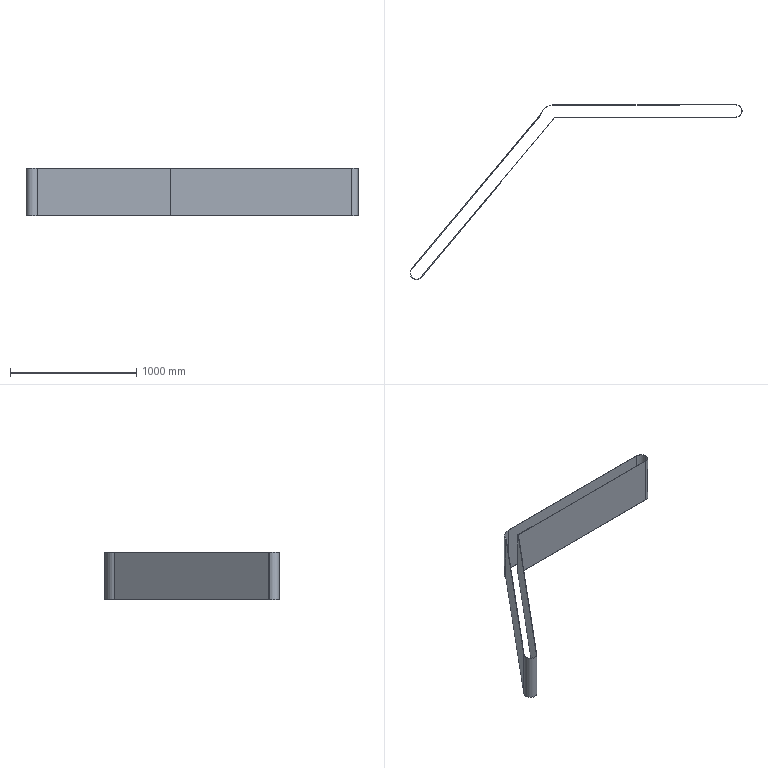Part | STEP file | Copy of PART1V11 | 1 solid | 18 faces | box 2633 x 1388 x 378 mm | volume 7453727 mm3 | plane 10 | cylinder 8 | commonest cylinder face diameters 97.16 x2 103.16 x2 97.182 x1 103.182 x1 212.439 x1 218.439 x1
STEP:
#1=CARTESIAN_POINT('',(0.,0.,0.));
#2=DIRECTION('',(0.,0.,1.));
#3=DIRECTION('',(1.,0.,0.));
#4=AXIS2_PLACEMENT_3D('',#1,#2,#3);
#5=CARTESIAN_POINT('',(472.127,652.827,-378.));
#6=VERTEX_POINT('',#5);
#7=CARTESIAN_POINT('',(472.127,652.827,0.));
#8=VERTEX_POINT('',#7);
#9=CARTESIAN_POINT('',(472.127,652.827,-378.));
#10=DIRECTION('',(0.,0.,1.));
#11=VECTOR('',#10,1.);
#12=LINE('',#9,#11);
#13=CARTESIAN_POINT('',(472.206,604.247,-378.));
#14=DIRECTION('',(0.,0.,1.));
#15=DIRECTION('',(1.,0.,0.));
#16=AXIS2_PLACEMENT_3D('',#13,#14,#15);
#17=CYLINDRICAL_SURFACE('',#16,48.58);
#18=CARTESIAN_POINT('',(1.572,0.));
#19=DIRECTION('',(0.,1.));
#20=VECTOR('',#19,1.);
#21=LINE('',#18,#20);
#22=(GEOMETRIC_REPRESENTATION_CONTEXT(2)PARAMETRIC_REPRESENTATION_CONTEXT()REPRESENTATION_CONTEXT('',''));
#23=DEFINITIONAL_REPRESENTATION('',(#21),#22);
#24=PCURVE('',#17,#23);
#25=CARTESIAN_POINT('',(472.127,652.827,-378.));
#26=DIRECTION('',(-0.001617,1.,0.));
#27=DIRECTION('',(-1.,-0.001617,0.));
#28=AXIS2_PLACEMENT_3D('',#25,#26,#27);
#29=PLANE('',#28);
#30=CARTESIAN_POINT('',(0.,0.));
#31=DIRECTION('',(0.,1.));
#32=VECTOR('',#31,1.);
#33=LINE('',#30,#32);
#34=(GEOMETRIC_REPRESENTATION_CONTEXT(2)PARAMETRIC_REPRESENTATION_CONTEXT()REPRESENTATION_CONTEXT('',''));
#35=DEFINITIONAL_REPRESENTATION('',(#33),#34);
#36=PCURVE('',#29,#35);
#37=SURFACE_CURVE('',#12,(#24,#36),.PCURVE_S1.);
#38=EDGE_CURVE('',#6,#8,#37,.T.);
#39=ORIENTED_EDGE('',*,*,#38,.T.);
#40=CARTESIAN_POINT('',(520.786,604.247,0.));
#41=VERTEX_POINT('',#40);
#42=CARTESIAN_POINT('',(472.206,604.247,0.));
#43=DIRECTION('',(0.,0.,1.));
#44=DIRECTION('',(1.,0.,0.));
#45=AXIS2_PLACEMENT_3D('',#42,#43,#44);
#46=CIRCLE('',#45,48.58);
#47=CARTESIAN_POINT('',(0.,378.));
#48=DIRECTION('',(1.,0.));
#49=VECTOR('',#48,1.);
#50=LINE('',#47,#49);
#51=(GEOMETRIC_REPRESENTATION_CONTEXT(2)PARAMETRIC_REPRESENTATION_CONTEXT()REPRESENTATION_CONTEXT('',''));
#52=DEFINITIONAL_REPRESENTATION('',(#50),#51);
#53=PCURVE('',#17,#52);
#54=CARTESIAN_POINT('',(-2057.802,-680.936,0.));
#55=DIRECTION('',(0.,0.,1.));
#56=DIRECTION('',(1.,0.,0.));
#57=AXIS2_PLACEMENT_3D('',#54,#55,#56);
#58=PLANE('',#57);
#59=CARTESIAN_POINT('',(2530.008,1285.182));
#60=DIRECTION('',(1.,0.));
#61=AXIS2_PLACEMENT_2D('',#59,#60);
#62=CIRCLE('',#61,48.58);
#63=(GEOMETRIC_REPRESENTATION_CONTEXT(2)PARAMETRIC_REPRESENTATION_CONTEXT()REPRESENTATION_CONTEXT('',''));
#64=DEFINITIONAL_REPRESENTATION('',(#62),#63);
#65=PCURVE('',#58,#64);
#66=SURFACE_CURVE('',#46,(#53,#65),.PCURVE_S1.);
#67=EDGE_CURVE('',#41,#8,#66,.T.);
#68=ORIENTED_EDGE('',*,*,#67,.F.);
#69=CARTESIAN_POINT('',(520.786,604.247,-378.));
#70=VERTEX_POINT('',#69);
#71=CARTESIAN_POINT('',(520.786,604.247,-378.));
#72=DIRECTION('',(0.,0.,1.));
#73=VECTOR('',#72,1.);
#74=LINE('',#71,#73);
#75=CARTESIAN_POINT('',(0.,0.));
#76=DIRECTION('',(0.,1.));
#77=VECTOR('',#76,1.);
#78=LINE('',#75,#77);
#79=(GEOMETRIC_REPRESENTATION_CONTEXT(2)PARAMETRIC_REPRESENTATION_CONTEXT()REPRESENTATION_CONTEXT('',''));
#80=DEFINITIONAL_REPRESENTATION('',(#78),#79);
#81=PCURVE('',#17,#80);
#82=CARTESIAN_POINT('',(472.206,604.247,-378.));
#83=DIRECTION('',(0.,0.,1.));
#84=DIRECTION('',(1.,0.,0.));
#85=AXIS2_PLACEMENT_3D('',#82,#83,#84);
#86=CYLINDRICAL_SURFACE('',#85,48.58);
#87=CARTESIAN_POINT('',(6.283,0.));
#88=DIRECTION('',(0.,1.));
#89=VECTOR('',#88,1.);
#90=LINE('',#87,#89);
#91=(GEOMETRIC_REPRESENTATION_CONTEXT(2)PARAMETRIC_REPRESENTATION_CONTEXT()REPRESENTATION_CONTEXT('',''));
#92=DEFINITIONAL_REPRESENTATION('',(#90),#91);
#93=PCURVE('',#86,#92);
#94=SURFACE_CURVE('',#74,(#81,#93),.PCURVE_S1.);
#95=EDGE_CURVE('',#70,#41,#94,.T.);
#96=ORIENTED_EDGE('',*,*,#95,.F.);
#97=CARTESIAN_POINT('',(472.206,604.247,-378.));
#98=DIRECTION('',(0.,0.,1.));
#99=DIRECTION('',(1.,0.,0.));
#100=AXIS2_PLACEMENT_3D('',#97,#98,#99);
#101=CIRCLE('',#100,48.58);
#102=CARTESIAN_POINT('',(0.,0.));
#103=DIRECTION('',(1.,0.));
#104=VECTOR('',#103,1.);
#105=LINE('',#102,#104);
#106=(GEOMETRIC_REPRESENTATION_CONTEXT(2)PARAMETRIC_REPRESENTATION_CONTEXT()REPRESENTATION_CONTEXT('',''));
#107=DEFINITIONAL_REPRESENTATION('',(#105),#106);
#108=PCURVE('',#17,#107);
#109=CARTESIAN_POINT('',(-2057.802,-680.936,-378.));
#110=DIRECTION('',(0.,0.,1.));
#111=DIRECTION('',(1.,0.,0.));
#112=AXIS2_PLACEMENT_3D('',#109,#110,#111);
#113=PLANE('',#112);
#114=CARTESIAN_POINT('',(2530.008,1285.182));
#115=DIRECTION('',(1.,0.));
#116=AXIS2_PLACEMENT_2D('',#114,#115);
#117=CIRCLE('',#116,48.58);
#118=(GEOMETRIC_REPRESENTATION_CONTEXT(2)PARAMETRIC_REPRESENTATION_CONTEXT()REPRESENTATION_CONTEXT('',''));
#119=DEFINITIONAL_REPRESENTATION('',(#117),#118);
#120=PCURVE('',#113,#119);
#121=SURFACE_CURVE('',#101,(#108,#120),.PCURVE_S1.);
#122=EDGE_CURVE('',#70,#6,#121,.T.);
#123=ORIENTED_EDGE('',*,*,#122,.T.);
#124=EDGE_LOOP('',(#39,#68,#96,#123));
#125=FACE_BOUND('',#124,.F.);
#126=ADVANCED_FACE('',(#125),#17,.F.);
#127=CARTESIAN_POINT('',(472.208,552.667,-378.));
#128=VERTEX_POINT('',#127);
#129=CARTESIAN_POINT('',(523.786,604.247,-378.));
#130=VERTEX_POINT('',#129);
#131=CARTESIAN_POINT('',(472.206,604.247,-378.));
#132=DIRECTION('',(0.,0.,1.));
#133=DIRECTION('',(1.,0.,0.));
#134=AXIS2_PLACEMENT_3D('',#131,#132,#133);
#135=CIRCLE('',#134,51.58);
#136=CARTESIAN_POINT('',(472.206,604.247,-378.));
#137=DIRECTION('',(0.,0.,1.));
#138=DIRECTION('',(1.,0.,0.));
#139=AXIS2_PLACEMENT_3D('',#136,#137,#138);
#140=CYLINDRICAL_SURFACE('',#139,51.58);
#141=CARTESIAN_POINT('',(0.,0.));
#142=DIRECTION('',(1.,0.));
#143=VECTOR('',#142,1.);
#144=LINE('',#141,#143);
#145=(GEOMETRIC_REPRESENTATION_CONTEXT(2)PARAMETRIC_REPRESENTATION_CONTEXT()REPRESENTATION_CONTEXT('',''));
#146=DEFINITIONAL_REPRESENTATION('',(#144),#145);
#147=PCURVE('',#140,#146);
#148=CARTESIAN_POINT('',(2530.008,1285.182));
#149=DIRECTION('',(1.,0.));
#150=AXIS2_PLACEMENT_2D('',#148,#149);
#151=CIRCLE('',#150,51.58);
#152=(GEOMETRIC_REPRESENTATION_CONTEXT(2)PARAMETRIC_REPRESENTATION_CONTEXT()REPRESENTATION_CONTEXT('',''));
#153=DEFINITIONAL_REPRESENTATION('',(#151),#152);
#154=PCURVE('',#113,#153);
#155=SURFACE_CURVE('',#135,(#147,#154),.PCURVE_S1.);
#156=EDGE_CURVE('',#128,#130,#155,.T.);
#157=ORIENTED_EDGE('',*,*,#156,.T.);
#158=CARTESIAN_POINT('',(523.786,604.247,0.));
#159=VERTEX_POINT('',#158);
#160=CARTESIAN_POINT('',(523.786,604.247,-378.));
#161=DIRECTION('',(0.,0.,1.));
#162=VECTOR('',#161,1.);
#163=LINE('',#160,#162);
#164=CARTESIAN_POINT('',(6.283,0.));
#165=DIRECTION('',(0.,1.));
#166=VECTOR('',#165,1.);
#167=LINE('',#164,#166);
#168=(GEOMETRIC_REPRESENTATION_CONTEXT(2)PARAMETRIC_REPRESENTATION_CONTEXT()REPRESENTATION_CONTEXT('',''));
#169=DEFINITIONAL_REPRESENTATION('',(#167),#168);
#170=PCURVE('',#140,#169);
#171=CARTESIAN_POINT('',(472.206,604.247,-378.));
#172=DIRECTION('',(0.,0.,1.));
#173=DIRECTION('',(1.,0.,0.));
#174=AXIS2_PLACEMENT_3D('',#171,#172,#173);
#175=CYLINDRICAL_SURFACE('',#174,51.58);
#176=CARTESIAN_POINT('',(0.,0.));
#177=DIRECTION('',(0.,1.));
#178=VECTOR('',#177,1.);
#179=LINE('',#176,#178);
#180=(GEOMETRIC_REPRESENTATION_CONTEXT(2)PARAMETRIC_REPRESENTATION_CONTEXT()REPRESENTATION_CONTEXT('',''));
#181=DEFINITIONAL_REPRESENTATION('',(#179),#180);
#182=PCURVE('',#175,#181);
#183=SURFACE_CURVE('',#163,(#170,#182),.PCURVE_S1.);
#184=EDGE_CURVE('',#130,#159,#183,.T.);
#185=ORIENTED_EDGE('',*,*,#184,.T.);
#186=CARTESIAN_POINT('',(472.208,552.667,0.));
#187=VERTEX_POINT('',#186);
#188=CARTESIAN_POINT('',(472.206,604.247,0.));
#189=DIRECTION('',(0.,0.,1.));
#190=DIRECTION('',(1.,0.,0.));
#191=AXIS2_PLACEMENT_3D('',#188,#189,#190);
#192=CIRCLE('',#191,51.58);
#193=CARTESIAN_POINT('',(0.,378.));
#194=DIRECTION('',(1.,0.));
#195=VECTOR('',#194,1.);
#196=LINE('',#193,#195);
#197=(GEOMETRIC_REPRESENTATION_CONTEXT(2)PARAMETRIC_REPRESENTATION_CONTEXT()REPRESENTATION_CONTEXT('',''));
#198=DEFINITIONAL_REPRESENTATION('',(#196),#197);
#199=PCURVE('',#140,#198);
#200=CARTESIAN_POINT('',(2530.008,1285.182));
#201=DIRECTION('',(1.,0.));
#202=AXIS2_PLACEMENT_2D('',#200,#201);
#203=CIRCLE('',#202,51.58);
#204=(GEOMETRIC_REPRESENTATION_CONTEXT(2)PARAMETRIC_REPRESENTATION_CONTEXT()REPRESENTATION_CONTEXT('',''));
#205=DEFINITIONAL_REPRESENTATION('',(#203),#204);
#206=PCURVE('',#58,#205);
#207=SURFACE_CURVE('',#192,(#199,#206),.PCURVE_S1.);
#208=EDGE_CURVE('',#187,#159,#207,.T.);
#209=ORIENTED_EDGE('',*,*,#208,.F.);
#210=CARTESIAN_POINT('',(472.208,552.667,-378.));
#211=DIRECTION('',(0.,0.,1.));
#212=VECTOR('',#211,1.);
#213=LINE('',#210,#212);
#214=CARTESIAN_POINT('',(4.712,0.));
#215=DIRECTION('',(0.,1.));
#216=VECTOR('',#215,1.);
#217=LINE('',#214,#216);
#218=(GEOMETRIC_REPRESENTATION_CONTEXT(2)PARAMETRIC_REPRESENTATION_CONTEXT()REPRESENTATION_CONTEXT('',''));
#219=DEFINITIONAL_REPRESENTATION('',(#217),#218);
#220=PCURVE('',#140,#219);
#221=CARTESIAN_POINT('',(472.208,552.667,-378.));
#222=DIRECTION('',(0.001617,-1.,0.));
#223=DIRECTION('',(1.,0.001617,0.));
#224=AXIS2_PLACEMENT_3D('',#221,#222,#223);
#225=PLANE('',#224);
#226=CARTESIAN_POINT('',(0.,0.));
#227=DIRECTION('',(0.,1.));
#228=VECTOR('',#227,1.);
#229=LINE('',#226,#228);
#230=(GEOMETRIC_REPRESENTATION_CONTEXT(2)PARAMETRIC_REPRESENTATION_CONTEXT()REPRESENTATION_CONTEXT('',''));
#231=DEFINITIONAL_REPRESENTATION('',(#229),#230);
#232=PCURVE('',#225,#231);
#233=SURFACE_CURVE('',#213,(#220,#232),.PCURVE_S1.);
#234=EDGE_CURVE('',#128,#187,#233,.T.);
#235=ORIENTED_EDGE('',*,*,#234,.F.);
#236=EDGE_LOOP('',(#157,#185,#209,#235));
#237=FACE_BOUND('',#236,.T.);
#238=ADVANCED_FACE('',(#237),#140,.T.);
#239=CARTESIAN_POINT('',(-2097.377,-647.838,0.));
#240=VERTEX_POINT('',#239);
#241=CARTESIAN_POINT('',(-2018.228,-714.034,0.));
#242=VERTEX_POINT('',#241);
#243=CARTESIAN_POINT('',(-2057.802,-680.936,0.));
#244=DIRECTION('',(0.,0.,1.));
#245=DIRECTION('',(1.,0.,0.));
#246=AXIS2_PLACEMENT_3D('',#243,#244,#245);
#247=CIRCLE('',#246,51.591);
#248=CARTESIAN_POINT('',(-2057.802,-680.936,-378.));
#249=DIRECTION('',(0.,0.,1.));
#250=DIRECTION('',(1.,0.,0.));
#251=AXIS2_PLACEMENT_3D('',#248,#249,#250);
#252=CYLINDRICAL_SURFACE('',#251,51.591);
#253=CARTESIAN_POINT('',(0.,378.));
#254=DIRECTION('',(1.,0.));
#255=VECTOR('',#254,1.);
#256=LINE('',#253,#255);
#257=(GEOMETRIC_REPRESENTATION_CONTEXT(2)PARAMETRIC_REPRESENTATION_CONTEXT()REPRESENTATION_CONTEXT('',''));
#258=DEFINITIONAL_REPRESENTATION('',(#256),#257);
#259=PCURVE('',#252,#258);
#260=CARTESIAN_POINT('',(0.,0.));
#261=DIRECTION('',(1.,0.));
#262=AXIS2_PLACEMENT_2D('',#260,#261);
#263=CIRCLE('',#262,51.591);
#264=(GEOMETRIC_REPRESENTATION_CONTEXT(2)PARAMETRIC_REPRESENTATION_CONTEXT()REPRESENTATION_CONTEXT('',''));
#265=DEFINITIONAL_REPRESENTATION('',(#263),#264);
#266=PCURVE('',#58,#265);
#267=SURFACE_CURVE('',#247,(#259,#266),.PCURVE_S1.);
#268=EDGE_CURVE('',#240,#242,#267,.T.);
#269=ORIENTED_EDGE('',*,*,#268,.F.);
#270=CARTESIAN_POINT('',(-2097.377,-647.838,-378.));
#271=VERTEX_POINT('',#270);
#272=CARTESIAN_POINT('',(-2097.377,-647.838,-378.));
#273=DIRECTION('',(0.,0.,1.));
#274=VECTOR('',#273,1.);
#275=LINE('',#272,#274);
#276=CARTESIAN_POINT('',(2.445,0.));
#277=DIRECTION('',(0.,1.));
#278=VECTOR('',#277,1.);
#279=LINE('',#276,#278);
#280=(GEOMETRIC_REPRESENTATION_CONTEXT(2)PARAMETRIC_REPRESENTATION_CONTEXT()REPRESENTATION_CONTEXT('',''));
#281=DEFINITIONAL_REPRESENTATION('',(#279),#280);
#282=PCURVE('',#252,#281);
#283=CARTESIAN_POINT('',(-2097.377,-647.838,-378.));
#284=DIRECTION('',(-0.7671,0.6415,0.));
#285=DIRECTION('',(-0.6415,-0.7671,0.));
#286=AXIS2_PLACEMENT_3D('',#283,#284,#285);
#287=PLANE('',#286);
#288=CARTESIAN_POINT('',(0.,0.));
#289=DIRECTION('',(0.,1.));
#290=VECTOR('',#289,1.);
#291=LINE('',#288,#290);
#292=(GEOMETRIC_REPRESENTATION_CONTEXT(2)PARAMETRIC_REPRESENTATION_CONTEXT()REPRESENTATION_CONTEXT('',''));
#293=DEFINITIONAL_REPRESENTATION('',(#291),#292);
#294=PCURVE('',#287,#293);
#295=SURFACE_CURVE('',#275,(#282,#294),.PCURVE_S1.);
#296=EDGE_CURVE('',#271,#240,#295,.T.);
#297=ORIENTED_EDGE('',*,*,#296,.F.);
#298=CARTESIAN_POINT('',(-2018.228,-714.034,-378.));
#299=VERTEX_POINT('',#298);
#300=CARTESIAN_POINT('',(-2057.802,-680.936,-378.));
#301=DIRECTION('',(0.,0.,1.));
#302=DIRECTION('',(1.,0.,0.));
#303=AXIS2_PLACEMENT_3D('',#300,#301,#302);
#304=CIRCLE('',#303,51.591);
#305=CARTESIAN_POINT('',(0.,0.));
#306=DIRECTION('',(1.,0.));
#307=VECTOR('',#306,1.);
#308=LINE('',#305,#307);
#309=(GEOMETRIC_REPRESENTATION_CONTEXT(2)PARAMETRIC_REPRESENTATION_CONTEXT()REPRESENTATION_CONTEXT('',''));
#310=DEFINITIONAL_REPRESENTATION('',(#308),#309);
#311=PCURVE('',#252,#310);
#312=CARTESIAN_POINT('',(0.,0.));
#313=DIRECTION('',(1.,0.));
#314=AXIS2_PLACEMENT_2D('',#312,#313);
#315=CIRCLE('',#314,51.591);
#316=(GEOMETRIC_REPRESENTATION_CONTEXT(2)PARAMETRIC_REPRESENTATION_CONTEXT()REPRESENTATION_CONTEXT('',''));
#317=DEFINITIONAL_REPRESENTATION('',(#315),#316);
#318=PCURVE('',#113,#317);
#319=SURFACE_CURVE('',#304,(#311,#318),.PCURVE_S1.);
#320=EDGE_CURVE('',#271,#299,#319,.T.);
#321=ORIENTED_EDGE('',*,*,#320,.T.);
#322=CARTESIAN_POINT('',(-2018.228,-714.034,-378.));
#323=DIRECTION('',(0.,0.,1.));
#324=VECTOR('',#323,1.);
#325=LINE('',#322,#324);
#326=CARTESIAN_POINT('',(5.587,0.));
#327=DIRECTION('',(0.,1.));
#328=VECTOR('',#327,1.);
#329=LINE('',#326,#328);
#330=(GEOMETRIC_REPRESENTATION_CONTEXT(2)PARAMETRIC_REPRESENTATION_CONTEXT()REPRESENTATION_CONTEXT('',''));
#331=DEFINITIONAL_REPRESENTATION('',(#329),#330);
#332=PCURVE('',#252,#331);
#333=CARTESIAN_POINT('',(-960.762,550.35,-378.));
#334=DIRECTION('',(0.7671,-0.6415,0.));
#335=DIRECTION('',(0.6415,0.7671,0.));
#336=AXIS2_PLACEMENT_3D('',#333,#334,#335);
#337=PLANE('',#336);
#338=CARTESIAN_POINT('',(-1648.303,0.));
#339=DIRECTION('',(0.,1.));
#340=VECTOR('',#339,1.);
#341=LINE('',#338,#340);
#342=(GEOMETRIC_REPRESENTATION_CONTEXT(2)PARAMETRIC_REPRESENTATION_CONTEXT()REPRESENTATION_CONTEXT('',''));
#343=DEFINITIONAL_REPRESENTATION('',(#341),#342);
#344=PCURVE('',#337,#343);
#345=SURFACE_CURVE('',#325,(#332,#344),.PCURVE_S1.);
#346=EDGE_CURVE('',#299,#242,#345,.T.);
#347=ORIENTED_EDGE('',*,*,#346,.T.);
#348=EDGE_LOOP('',(#269,#297,#321,#347));
#349=FACE_BOUND('',#348,.T.);
#350=ADVANCED_FACE('',(#349),#252,.T.);
#351=CARTESIAN_POINT('',(-1075.448,574.055,0.));
#352=VERTEX_POINT('',#351);
#353=CARTESIAN_POINT('',(-2097.377,-647.838,0.));
#354=DIRECTION('',(-0.6415,-0.7671,0.));
#355=VECTOR('',#354,1.);
#356=LINE('',#353,#355);
#357=CARTESIAN_POINT('',(0.,378.));
#358=DIRECTION('',(1.,0.));
#359=VECTOR('',#358,1.);
#360=LINE('',#357,#359);
#361=(GEOMETRIC_REPRESENTATION_CONTEXT(2)PARAMETRIC_REPRESENTATION_CONTEXT()REPRESENTATION_CONTEXT('',''));
#362=DEFINITIONAL_REPRESENTATION('',(#360),#361);
#363=PCURVE('',#287,#362);
#364=CARTESIAN_POINT('',(-39.574,33.098));
#365=DIRECTION('',(-0.6415,-0.7671));
#366=VECTOR('',#365,1.);
#367=LINE('',#364,#366);
#368=(GEOMETRIC_REPRESENTATION_CONTEXT(2)PARAMETRIC_REPRESENTATION_CONTEXT()REPRESENTATION_CONTEXT('',''));
#369=DEFINITIONAL_REPRESENTATION('',(#367),#368);
#370=PCURVE('',#58,#369);
#371=SURFACE_CURVE('',#356,(#363,#370),.PCURVE_S1.);
#372=EDGE_CURVE('',#352,#240,#371,.T.);
#373=ORIENTED_EDGE('',*,*,#372,.F.);
#374=CARTESIAN_POINT('',(-1075.448,574.055,-378.));
#375=VERTEX_POINT('',#374);
#376=CARTESIAN_POINT('',(-1075.448,574.055,-378.));
#377=DIRECTION('',(0.,0.,1.));
#378=VECTOR('',#377,1.);
#379=LINE('',#376,#378);
#380=CARTESIAN_POINT('',(-1592.909,0.));
#381=DIRECTION('',(0.,1.));
#382=VECTOR('',#381,1.);
#383=LINE('',#380,#382);
#384=(GEOMETRIC_REPRESENTATION_CONTEXT(2)PARAMETRIC_REPRESENTATION_CONTEXT()REPRESENTATION_CONTEXT('',''));
#385=DEFINITIONAL_REPRESENTATION('',(#383),#384);
#386=PCURVE('',#287,#385);
#387=CARTESIAN_POINT('',(-970.367,544.275,-378.));
#388=DIRECTION('',(0.,0.,1.));
#389=DIRECTION('',(1.,0.,0.));
#390=AXIS2_PLACEMENT_3D('',#387,#388,#389);
#391=CYLINDRICAL_SURFACE('',#390,109.22);
#392=CARTESIAN_POINT('',(2.865,0.));
#393=DIRECTION('',(0.,1.));
#394=VECTOR('',#393,1.);
#395=LINE('',#392,#394);
#396=(GEOMETRIC_REPRESENTATION_CONTEXT(2)PARAMETRIC_REPRESENTATION_CONTEXT()REPRESENTATION_CONTEXT('',''));
#397=DEFINITIONAL_REPRESENTATION('',(#395),#396);
#398=PCURVE('',#391,#397);
#399=SURFACE_CURVE('',#379,(#386,#398),.PCURVE_S1.);
#400=EDGE_CURVE('',#375,#352,#399,.T.);
#401=ORIENTED_EDGE('',*,*,#400,.F.);
#402=CARTESIAN_POINT('',(-2097.377,-647.838,-378.));
#403=DIRECTION('',(-0.6415,-0.7671,0.));
#404=VECTOR('',#403,1.);
#405=LINE('',#402,#404);
#406=CARTESIAN_POINT('',(0.,0.));
#407=DIRECTION('',(1.,0.));
#408=VECTOR('',#407,1.);
#409=LINE('',#406,#408);
#410=(GEOMETRIC_REPRESENTATION_CONTEXT(2)PARAMETRIC_REPRESENTATION_CONTEXT()REPRESENTATION_CONTEXT('',''));
#411=DEFINITIONAL_REPRESENTATION('',(#409),#410);
#412=PCURVE('',#287,#411);
#413=CARTESIAN_POINT('',(-39.574,33.098));
#414=DIRECTION('',(-0.6415,-0.7671));
#415=VECTOR('',#414,1.);
#416=LINE('',#413,#415);
#417=(GEOMETRIC_REPRESENTATION_CONTEXT(2)PARAMETRIC_REPRESENTATION_CONTEXT()REPRESENTATION_CONTEXT('',''));
#418=DEFINITIONAL_REPRESENTATION('',(#416),#417);
#419=PCURVE('',#113,#418);
#420=SURFACE_CURVE('',#405,(#412,#419),.PCURVE_S1.);
#421=EDGE_CURVE('',#375,#271,#420,.T.);
#422=ORIENTED_EDGE('',*,*,#421,.T.);
#423=ORIENTED_EDGE('',*,*,#296,.T.);
#424=EDGE_LOOP('',(#373,#401,#422,#423));
#425=FACE_BOUND('',#424,.T.);
#426=ADVANCED_FACE('',(#425),#287,.T.);
#427=CARTESIAN_POINT('',(-970.543,653.495,0.));
#428=VERTEX_POINT('',#427);
#429=CARTESIAN_POINT('',(-970.367,544.275,0.));
#430=DIRECTION('',(0.,0.,1.));
#431=DIRECTION('',(1.,0.,0.));
#432=AXIS2_PLACEMENT_3D('',#429,#430,#431);
#433=CIRCLE('',#432,109.22);
#434=CARTESIAN_POINT('',(0.,378.));
#435=DIRECTION('',(1.,0.));
#436=VECTOR('',#435,1.);
#437=LINE('',#434,#436);
#438=(GEOMETRIC_REPRESENTATION_CONTEXT(2)PARAMETRIC_REPRESENTATION_CONTEXT()REPRESENTATION_CONTEXT('',''));
#439=DEFINITIONAL_REPRESENTATION('',(#437),#438);
#440=PCURVE('',#391,#439);
#441=CARTESIAN_POINT('',(1087.435,1225.211));
#442=DIRECTION('',(1.,0.));
#443=AXIS2_PLACEMENT_2D('',#441,#442);
#444=CIRCLE('',#443,109.22);
#445=(GEOMETRIC_REPRESENTATION_CONTEXT(2)PARAMETRIC_REPRESENTATION_CONTEXT()REPRESENTATION_CONTEXT('',''));
#446=DEFINITIONAL_REPRESENTATION('',(#444),#445);
#447=PCURVE('',#58,#446);
#448=SURFACE_CURVE('',#433,(#440,#447),.PCURVE_S1.);
#449=EDGE_CURVE('',#428,#352,#448,.T.);
#450=ORIENTED_EDGE('',*,*,#449,.F.);
#451=CARTESIAN_POINT('',(-970.543,653.495,-378.));
#452=VERTEX_POINT('',#451);
#453=CARTESIAN_POINT('',(-970.543,653.495,-378.));
#454=DIRECTION('',(0.,0.,1.));
#455=VECTOR('',#454,1.);
#456=LINE('',#453,#455);
#457=CARTESIAN_POINT('',(1.572,0.));
#458=DIRECTION('',(0.,1.));
#459=VECTOR('',#458,1.);
#460=LINE('',#457,#459);
#461=(GEOMETRIC_REPRESENTATION_CONTEXT(2)PARAMETRIC_REPRESENTATION_CONTEXT()REPRESENTATION_CONTEXT('',''));
#462=DEFINITIONAL_REPRESENTATION('',(#460),#461);
#463=PCURVE('',#391,#462);
#464=CARTESIAN_POINT('',(472.122,655.827,-378.));
#465=DIRECTION('',(-0.001617,1.,0.));
#466=DIRECTION('',(-1.,-0.001617,0.));
#467=AXIS2_PLACEMENT_3D('',#464,#465,#466);
#468=PLANE('',#467);
#469=CARTESIAN_POINT('',(1442.668,0.));
#470=DIRECTION('',(0.,1.));
#471=VECTOR('',#470,1.);
#472=LINE('',#469,#471);
#473=(GEOMETRIC_REPRESENTATION_CONTEXT(2)PARAMETRIC_REPRESENTATION_CONTEXT()REPRESENTATION_CONTEXT('',''));
#474=DEFINITIONAL_REPRESENTATION('',(#472),#473);
#475=PCURVE('',#468,#474);
#476=SURFACE_CURVE('',#456,(#463,#475),.PCURVE_S1.);
#477=EDGE_CURVE('',#452,#428,#476,.T.);
#478=ORIENTED_EDGE('',*,*,#477,.F.);
#479=CARTESIAN_POINT('',(-970.367,544.275,-378.));
#480=DIRECTION('',(0.,0.,1.));
#481=DIRECTION('',(1.,0.,0.));
#482=AXIS2_PLACEMENT_3D('',#479,#480,#481);
#483=CIRCLE('',#482,109.22);
#484=CARTESIAN_POINT('',(0.,0.));
#485=DIRECTION('',(1.,0.));
#486=VECTOR('',#485,1.);
#487=LINE('',#484,#486);
#488=(GEOMETRIC_REPRESENTATION_CONTEXT(2)PARAMETRIC_REPRESENTATION_CONTEXT()REPRESENTATION_CONTEXT('',''));
#489=DEFINITIONAL_REPRESENTATION('',(#487),#488);
#490=PCURVE('',#391,#489);
#491=CARTESIAN_POINT('',(1087.435,1225.211));
#492=DIRECTION('',(1.,0.));
#493=AXIS2_PLACEMENT_2D('',#491,#492);
#494=CIRCLE('',#493,109.22);
#495=(GEOMETRIC_REPRESENTATION_CONTEXT(2)PARAMETRIC_REPRESENTATION_CONTEXT()REPRESENTATION_CONTEXT('',''));
#496=DEFINITIONAL_REPRESENTATION('',(#494),#495);
#497=PCURVE('',#113,#496);
#498=SURFACE_CURVE('',#483,(#490,#497),.PCURVE_S1.);
#499=EDGE_CURVE('',#452,#375,#498,.T.);
#500=ORIENTED_EDGE('',*,*,#499,.T.);
#501=ORIENTED_EDGE('',*,*,#400,.T.);
#502=EDGE_LOOP('',(#450,#478,#500,#501));
#503=FACE_BOUND('',#502,.T.);
#504=ADVANCED_FACE('',(#503),#391,.T.);
#505=CARTESIAN_POINT('',(472.122,655.827,0.));
#506=VERTEX_POINT('',#505);
#507=CARTESIAN_POINT('',(472.122,655.827,0.));
#508=DIRECTION('',(-1.,-0.001617,0.));
#509=VECTOR('',#508,1.);
#510=LINE('',#507,#509);
#511=CARTESIAN_POINT('',(0.,378.));
#512=DIRECTION('',(1.,0.));
#513=VECTOR('',#512,1.);
#514=LINE('',#511,#513);
#515=(GEOMETRIC_REPRESENTATION_CONTEXT(2)PARAMETRIC_REPRESENTATION_CONTEXT()REPRESENTATION_CONTEXT('',''));
#516=DEFINITIONAL_REPRESENTATION('',(#514),#515);
#517=PCURVE('',#468,#516);
#518=CARTESIAN_POINT('',(2529.925,1336.762));
#519=DIRECTION('',(-1.,-0.001617));
#520=VECTOR('',#519,1.);
#521=LINE('',#518,#520);
#522=(GEOMETRIC_REPRESENTATION_CONTEXT(2)PARAMETRIC_REPRESENTATION_CONTEXT()REPRESENTATION_CONTEXT('',''));
#523=DEFINITIONAL_REPRESENTATION('',(#521),#522);
#524=PCURVE('',#58,#523);
#525=SURFACE_CURVE('',#510,(#517,#524),.PCURVE_S1.);
#526=EDGE_CURVE('',#506,#428,#525,.T.);
#527=ORIENTED_EDGE('',*,*,#526,.F.);
#528=CARTESIAN_POINT('',(472.122,655.827,-378.));
#529=VERTEX_POINT('',#528);
#530=CARTESIAN_POINT('',(472.122,655.827,-378.));
#531=DIRECTION('',(0.,0.,1.));
#532=VECTOR('',#531,1.);
#533=LINE('',#530,#532);
#534=CARTESIAN_POINT('',(0.,0.));
#535=DIRECTION('',(0.,1.));
#536=VECTOR('',#535,1.);
#537=LINE('',#534,#536);
#538=(GEOMETRIC_REPRESENTATION_CONTEXT(2)PARAMETRIC_REPRESENTATION_CONTEXT()REPRESENTATION_CONTEXT('',''));
#539=DEFINITIONAL_REPRESENTATION('',(#537),#538);
#540=PCURVE('',#468,#539);
#541=CARTESIAN_POINT('',(1.572,0.));
#542=DIRECTION('',(0.,1.));
#543=VECTOR('',#542,1.);
#544=LINE('',#541,#543);
#545=(GEOMETRIC_REPRESENTATION_CONTEXT(2)PARAMETRIC_REPRESENTATION_CONTEXT()REPRESENTATION_CONTEXT('',''));
#546=DEFINITIONAL_REPRESENTATION('',(#544),#545);
#547=PCURVE('',#175,#546);
#548=SURFACE_CURVE('',#533,(#540,#547),.PCURVE_S1.);
#549=EDGE_CURVE('',#529,#506,#548,.T.);
#550=ORIENTED_EDGE('',*,*,#549,.F.);
#551=CARTESIAN_POINT('',(472.122,655.827,-378.));
#552=DIRECTION('',(-1.,-0.001617,0.));
#553=VECTOR('',#552,1.);
#554=LINE('',#551,#553);
#555=CARTESIAN_POINT('',(0.,0.));
#556=DIRECTION('',(1.,0.));
#557=VECTOR('',#556,1.);
#558=LINE('',#555,#557);
#559=(GEOMETRIC_REPRESENTATION_CONTEXT(2)PARAMETRIC_REPRESENTATION_CONTEXT()REPRESENTATION_CONTEXT('',''));
#560=DEFINITIONAL_REPRESENTATION('',(#558),#559);
#561=PCURVE('',#468,#560);
#562=CARTESIAN_POINT('',(2529.925,1336.762));
#563=DIRECTION('',(-1.,-0.001617));
#564=VECTOR('',#563,1.);
#565=LINE('',#562,#564);
#566=(GEOMETRIC_REPRESENTATION_CONTEXT(2)PARAMETRIC_REPRESENTATION_CONTEXT()REPRESENTATION_CONTEXT('',''));
#567=DEFINITIONAL_REPRESENTATION('',(#565),#566);
#568=PCURVE('',#113,#567);
#569=SURFACE_CURVE('',#554,(#561,#568),.PCURVE_S1.);
#570=EDGE_CURVE('',#529,#452,#569,.T.);
#571=ORIENTED_EDGE('',*,*,#570,.T.);
#572=ORIENTED_EDGE('',*,*,#477,.T.);
#573=EDGE_LOOP('',(#527,#550,#571,#572));
#574=FACE_BOUND('',#573,.T.);
#575=ADVANCED_FACE('',(#574),#468,.T.);
#576=ORIENTED_EDGE('',*,*,#184,.F.);
#577=CARTESIAN_POINT('',(472.206,604.247,-378.));
#578=DIRECTION('',(0.,0.,1.));
#579=DIRECTION('',(1.,0.,0.));
#580=AXIS2_PLACEMENT_3D('',#577,#578,#579);
#581=CIRCLE('',#580,51.58);
#582=CARTESIAN_POINT('',(0.,0.));
#583=DIRECTION('',(1.,0.));
#584=VECTOR('',#583,1.);
#585=LINE('',#582,#584);
#586=(GEOMETRIC_REPRESENTATION_CONTEXT(2)PARAMETRIC_REPRESENTATION_CONTEXT()REPRESENTATION_CONTEXT('',''));
#587=DEFINITIONAL_REPRESENTATION('',(#585),#586);
#588=PCURVE('',#175,#587);
#589=CARTESIAN_POINT('',(2530.008,1285.182));
#590=DIRECTION('',(1.,0.));
#591=AXIS2_PLACEMENT_2D('',#589,#590);
#592=CIRCLE('',#591,51.58);
#593=(GEOMETRIC_REPRESENTATION_CONTEXT(2)PARAMETRIC_REPRESENTATION_CONTEXT()REPRESENTATION_CONTEXT('',''));
#594=DEFINITIONAL_REPRESENTATION('',(#592),#593);
#595=PCURVE('',#113,#594);
#596=SURFACE_CURVE('',#581,(#588,#595),.PCURVE_S1.);
#597=EDGE_CURVE('',#130,#529,#596,.T.);
#598=ORIENTED_EDGE('',*,*,#597,.T.);
#599=ORIENTED_EDGE('',*,*,#549,.T.);
#600=CARTESIAN_POINT('',(472.206,604.247,0.));
#601=DIRECTION('',(0.,0.,1.));
#602=DIRECTION('',(1.,0.,0.));
#603=AXIS2_PLACEMENT_3D('',#600,#601,#602);
#604=CIRCLE('',#603,51.58);
#605=CARTESIAN_POINT('',(0.,378.));
#606=DIRECTION('',(1.,0.));
#607=VECTOR('',#606,1.);
#608=LINE('',#605,#607);
#609=(GEOMETRIC_REPRESENTATION_CONTEXT(2)PARAMETRIC_REPRESENTATION_CONTEXT()REPRESENTATION_CONTEXT('',''));
#610=DEFINITIONAL_REPRESENTATION('',(#608),#609);
#611=PCURVE('',#175,#610);
#612=CARTESIAN_POINT('',(2530.008,1285.182));
#613=DIRECTION('',(1.,0.));
#614=AXIS2_PLACEMENT_2D('',#612,#613);
#615=CIRCLE('',#614,51.58);
#616=(GEOMETRIC_REPRESENTATION_CONTEXT(2)PARAMETRIC_REPRESENTATION_CONTEXT()REPRESENTATION_CONTEXT('',''));
#617=DEFINITIONAL_REPRESENTATION('',(#615),#616);
#618=PCURVE('',#58,#617);
#619=SURFACE_CURVE('',#604,(#611,#618),.PCURVE_S1.);
#620=EDGE_CURVE('',#159,#506,#619,.T.);
#621=ORIENTED_EDGE('',*,*,#620,.F.);
#622=EDGE_LOOP('',(#576,#598,#599,#621));
#623=FACE_BOUND('',#622,.T.);
#624=ADVANCED_FACE('',(#623),#175,.T.);
#625=CARTESIAN_POINT('',(-960.762,550.35,0.));
#626=VERTEX_POINT('',#625);
#627=CARTESIAN_POINT('',(472.208,552.667,0.));
#628=DIRECTION('',(1.,0.001617,0.));
#629=VECTOR('',#628,1.);
#630=LINE('',#627,#629);
#631=CARTESIAN_POINT('',(0.,378.));
#632=DIRECTION('',(1.,0.));
#633=VECTOR('',#632,1.);
#634=LINE('',#631,#633);
#635=(GEOMETRIC_REPRESENTATION_CONTEXT(2)PARAMETRIC_REPRESENTATION_CONTEXT()REPRESENTATION_CONTEXT('',''));
#636=DEFINITIONAL_REPRESENTATION('',(#634),#635);
#637=PCURVE('',#225,#636);
#638=CARTESIAN_POINT('',(2530.01,1233.602));
#639=DIRECTION('',(1.,0.001617));
#640=VECTOR('',#639,1.);
#641=LINE('',#638,#640);
#642=(GEOMETRIC_REPRESENTATION_CONTEXT(2)PARAMETRIC_REPRESENTATION_CONTEXT()REPRESENTATION_CONTEXT('',''));
#643=DEFINITIONAL_REPRESENTATION('',(#641),#642);
#644=PCURVE('',#58,#643);
#645=SURFACE_CURVE('',#630,(#637,#644),.PCURVE_S1.);
#646=EDGE_CURVE('',#626,#187,#645,.T.);
#647=ORIENTED_EDGE('',*,*,#646,.F.);
#648=CARTESIAN_POINT('',(-960.762,550.35,-378.));
#649=VERTEX_POINT('',#648);
#650=CARTESIAN_POINT('',(-960.762,550.35,-378.));
#651=DIRECTION('',(0.,0.,1.));
#652=VECTOR('',#651,1.);
#653=LINE('',#650,#652);
#654=CARTESIAN_POINT('',(-1432.972,0.));
#655=DIRECTION('',(0.,1.));
#656=VECTOR('',#655,1.);
#657=LINE('',#654,#656);
#658=(GEOMETRIC_REPRESENTATION_CONTEXT(2)PARAMETRIC_REPRESENTATION_CONTEXT()REPRESENTATION_CONTEXT('',''));
#659=DEFINITIONAL_REPRESENTATION('',(#657),#658);
#660=PCURVE('',#225,#659);
#661=CARTESIAN_POINT('',(0.,0.));
#662=DIRECTION('',(0.,1.));
#663=VECTOR('',#662,1.);
#664=LINE('',#661,#663);
#665=(GEOMETRIC_REPRESENTATION_CONTEXT(2)PARAMETRIC_REPRESENTATION_CONTEXT()REPRESENTATION_CONTEXT('',''));
#666=DEFINITIONAL_REPRESENTATION('',(#664),#665);
#667=PCURVE('',#337,#666);
#668=SURFACE_CURVE('',#653,(#660,#667),.PCURVE_S1.);
#669=EDGE_CURVE('',#649,#626,#668,.T.);
#670=ORIENTED_EDGE('',*,*,#669,.F.);
#671=CARTESIAN_POINT('',(472.208,552.667,-378.));
#672=DIRECTION('',(1.,0.001617,0.));
#673=VECTOR('',#672,1.);
#674=LINE('',#671,#673);
#675=CARTESIAN_POINT('',(0.,0.));
#676=DIRECTION('',(1.,0.));
#677=VECTOR('',#676,1.);
#678=LINE('',#675,#677);
#679=(GEOMETRIC_REPRESENTATION_CONTEXT(2)PARAMETRIC_REPRESENTATION_CONTEXT()REPRESENTATION_CONTEXT('',''));
#680=DEFINITIONAL_REPRESENTATION('',(#678),#679);
#681=PCURVE('',#225,#680);
#682=CARTESIAN_POINT('',(2530.01,1233.602));
#683=DIRECTION('',(1.,0.001617));
#684=VECTOR('',#683,1.);
#685=LINE('',#682,#684);
#686=(GEOMETRIC_REPRESENTATION_CONTEXT(2)PARAMETRIC_REPRESENTATION_CONTEXT()REPRESENTATION_CONTEXT('',''));
#687=DEFINITIONAL_REPRESENTATION('',(#685),#686);
#688=PCURVE('',#113,#687);
#689=SURFACE_CURVE('',#674,(#681,#688),.PCURVE_S1.);
#690=EDGE_CURVE('',#649,#128,#689,.T.);
#691=ORIENTED_EDGE('',*,*,#690,.T.);
#692=ORIENTED_EDGE('',*,*,#234,.T.);
#693=EDGE_LOOP('',(#647,#670,#691,#692));
#694=FACE_BOUND('',#693,.T.);
#695=ADVANCED_FACE('',(#694),#225,.T.);
#696=CARTESIAN_POINT('',(-960.762,550.35,0.));
#697=DIRECTION('',(0.6415,0.7671,0.));
#698=VECTOR('',#697,1.);
#699=LINE('',#696,#698);
#700=CARTESIAN_POINT('',(0.,378.));
#701=DIRECTION('',(1.,0.));
#702=VECTOR('',#701,1.);
#703=LINE('',#700,#702);
#704=(GEOMETRIC_REPRESENTATION_CONTEXT(2)PARAMETRIC_REPRESENTATION_CONTEXT()REPRESENTATION_CONTEXT('',''));
#705=DEFINITIONAL_REPRESENTATION('',(#703),#704);
#706=PCURVE('',#337,#705);
#707=CARTESIAN_POINT('',(1097.04,1231.286));
#708=DIRECTION('',(0.6415,0.7671));
#709=VECTOR('',#708,1.);
#710=LINE('',#707,#709);
#711=(GEOMETRIC_REPRESENTATION_CONTEXT(2)PARAMETRIC_REPRESENTATION_CONTEXT()REPRESENTATION_CONTEXT('',''));
#712=DEFINITIONAL_REPRESENTATION('',(#710),#711);
#713=PCURVE('',#58,#712);
#714=SURFACE_CURVE('',#699,(#706,#713),.PCURVE_S1.);
#715=EDGE_CURVE('',#242,#626,#714,.T.);
#716=ORIENTED_EDGE('',*,*,#715,.F.);
#717=ORIENTED_EDGE('',*,*,#346,.F.);
#718=CARTESIAN_POINT('',(-960.762,550.35,-378.));
#719=DIRECTION('',(0.6415,0.7671,0.));
#720=VECTOR('',#719,1.);
#721=LINE('',#718,#720);
#722=CARTESIAN_POINT('',(0.,0.));
#723=DIRECTION('',(1.,0.));
#724=VECTOR('',#723,1.);
#725=LINE('',#722,#724);
#726=(GEOMETRIC_REPRESENTATION_CONTEXT(2)PARAMETRIC_REPRESENTATION_CONTEXT()REPRESENTATION_CONTEXT('',''));
#727=DEFINITIONAL_REPRESENTATION('',(#725),#726);
#728=PCURVE('',#337,#727);
#729=CARTESIAN_POINT('',(1097.04,1231.286));
#730=DIRECTION('',(0.6415,0.7671));
#731=VECTOR('',#730,1.);
#732=LINE('',#729,#731);
#733=(GEOMETRIC_REPRESENTATION_CONTEXT(2)PARAMETRIC_REPRESENTATION_CONTEXT()REPRESENTATION_CONTEXT('',''));
#734=DEFINITIONAL_REPRESENTATION('',(#732),#733);
#735=PCURVE('',#113,#734);
#736=SURFACE_CURVE('',#721,(#728,#735),.PCURVE_S1.);
#737=EDGE_CURVE('',#299,#649,#736,.T.);
#738=ORIENTED_EDGE('',*,*,#737,.T.);
#739=ORIENTED_EDGE('',*,*,#669,.T.);
#740=EDGE_LOOP('',(#716,#717,#738,#739));
#741=FACE_BOUND('',#740,.T.);
#742=ADVANCED_FACE('',(#741),#337,.T.);
#743=CARTESIAN_POINT('',(-2020.529,-712.109,-378.));
#744=VERTEX_POINT('',#743);
#745=CARTESIAN_POINT('',(-962.166,553.348,-378.));
#746=VERTEX_POINT('',#745);
#747=CARTESIAN_POINT('',(-962.166,553.348,-378.));
#748=DIRECTION('',(0.6415,0.7671,0.));
#749=VECTOR('',#748,1.);
#750=LINE('',#747,#749);
#751=CARTESIAN_POINT('',(1095.637,1234.284));
#752=DIRECTION('',(0.6415,0.7671));
#753=VECTOR('',#752,1.);
#754=LINE('',#751,#753);
#755=(GEOMETRIC_REPRESENTATION_CONTEXT(2)PARAMETRIC_REPRESENTATION_CONTEXT()REPRESENTATION_CONTEXT('',''));
#756=DEFINITIONAL_REPRESENTATION('',(#754),#755);
#757=PCURVE('',#113,#756);
#758=CARTESIAN_POINT('',(-962.166,553.348,-378.));
#759=DIRECTION('',(0.7671,-0.6415,0.));
#760=DIRECTION('',(0.6415,0.7671,0.));
#761=AXIS2_PLACEMENT_3D('',#758,#759,#760);
#762=PLANE('',#761);
#763=CARTESIAN_POINT('',(0.,0.));
#764=DIRECTION('',(1.,0.));
#765=VECTOR('',#764,1.);
#766=LINE('',#763,#765);
#767=(GEOMETRIC_REPRESENTATION_CONTEXT(2)PARAMETRIC_REPRESENTATION_CONTEXT()REPRESENTATION_CONTEXT('',''));
#768=DEFINITIONAL_REPRESENTATION('',(#766),#767);
#769=PCURVE('',#762,#768);
#770=SURFACE_CURVE('',#750,(#757,#769),.PCURVE_S1.);
#771=EDGE_CURVE('',#744,#746,#770,.T.);
#772=ORIENTED_EDGE('',*,*,#771,.T.);
#773=CARTESIAN_POINT('',(472.206,555.667,-378.));
#774=VERTEX_POINT('',#773);
#775=CARTESIAN_POINT('',(472.206,555.667,-378.));
#776=DIRECTION('',(1.,0.001617,0.));
#777=VECTOR('',#776,1.);
#778=LINE('',#775,#777);
#779=CARTESIAN_POINT('',(2530.008,1236.602));
#780=DIRECTION('',(1.,0.001617));
#781=VECTOR('',#780,1.);
#782=LINE('',#779,#781);
#783=(GEOMETRIC_REPRESENTATION_CONTEXT(2)PARAMETRIC_REPRESENTATION_CONTEXT()REPRESENTATION_CONTEXT('',''));
#784=DEFINITIONAL_REPRESENTATION('',(#782),#783);
#785=PCURVE('',#113,#784);
#786=CARTESIAN_POINT('',(472.206,555.667,-378.));
#787=DIRECTION('',(0.001617,-1.,0.));
#788=DIRECTION('',(1.,0.001617,0.));
#789=AXIS2_PLACEMENT_3D('',#786,#787,#788);
#790=PLANE('',#789);
#791=CARTESIAN_POINT('',(0.,0.));
#792=DIRECTION('',(1.,0.));
#793=VECTOR('',#792,1.);
#794=LINE('',#791,#793);
#795=(GEOMETRIC_REPRESENTATION_CONTEXT(2)PARAMETRIC_REPRESENTATION_CONTEXT()REPRESENTATION_CONTEXT('',''));
#796=DEFINITIONAL_REPRESENTATION('',(#794),#795);
#797=PCURVE('',#790,#796);
#798=SURFACE_CURVE('',#778,(#785,#797),.PCURVE_S1.);
#799=EDGE_CURVE('',#746,#774,#798,.T.);
#800=ORIENTED_EDGE('',*,*,#799,.T.);
#801=CARTESIAN_POINT('',(472.206,604.247,-378.));
#802=DIRECTION('',(0.,0.,1.));
#803=DIRECTION('',(1.,0.,0.));
#804=AXIS2_PLACEMENT_3D('',#801,#802,#803);
#805=CIRCLE('',#804,48.58);
#806=CARTESIAN_POINT('',(2530.008,1285.182));
#807=DIRECTION('',(1.,0.));
#808=AXIS2_PLACEMENT_2D('',#806,#807);
#809=CIRCLE('',#808,48.58);
#810=(GEOMETRIC_REPRESENTATION_CONTEXT(2)PARAMETRIC_REPRESENTATION_CONTEXT()REPRESENTATION_CONTEXT('',''));
#811=DEFINITIONAL_REPRESENTATION('',(#809),#810);
#812=PCURVE('',#113,#811);
#813=CARTESIAN_POINT('',(0.,0.));
#814=DIRECTION('',(1.,0.));
#815=VECTOR('',#814,1.);
#816=LINE('',#813,#815);
#817=(GEOMETRIC_REPRESENTATION_CONTEXT(2)PARAMETRIC_REPRESENTATION_CONTEXT()REPRESENTATION_CONTEXT('',''));
#818=DEFINITIONAL_REPRESENTATION('',(#816),#817);
#819=PCURVE('',#86,#818);
#820=SURFACE_CURVE('',#805,(#812,#819),.PCURVE_S1.);
#821=EDGE_CURVE('',#774,#70,#820,.T.);
#822=ORIENTED_EDGE('',*,*,#821,.T.);
#823=ORIENTED_EDGE('',*,*,#122,.T.);
#824=CARTESIAN_POINT('',(-970.539,650.495,-378.));
#825=VERTEX_POINT('',#824);
#826=CARTESIAN_POINT('',(472.127,652.827,-378.));
#827=DIRECTION('',(-1.,-0.001617,0.));
#828=VECTOR('',#827,1.);
#829=LINE('',#826,#828);
#830=CARTESIAN_POINT('',(2529.929,1333.762));
#831=DIRECTION('',(-1.,-0.001617));
#832=VECTOR('',#831,1.);
#833=LINE('',#830,#832);
#834=(GEOMETRIC_REPRESENTATION_CONTEXT(2)PARAMETRIC_REPRESENTATION_CONTEXT()REPRESENTATION_CONTEXT('',''));
#835=DEFINITIONAL_REPRESENTATION('',(#833),#834);
#836=PCURVE('',#113,#835);
#837=CARTESIAN_POINT('',(0.,0.));
#838=DIRECTION('',(1.,0.));
#839=VECTOR('',#838,1.);
#840=LINE('',#837,#839);
#841=(GEOMETRIC_REPRESENTATION_CONTEXT(2)PARAMETRIC_REPRESENTATION_CONTEXT()REPRESENTATION_CONTEXT('',''));
#842=DEFINITIONAL_REPRESENTATION('',(#840),#841);
#843=PCURVE('',#29,#842);
#844=SURFACE_CURVE('',#829,(#836,#843),.PCURVE_S1.);
#845=EDGE_CURVE('',#6,#825,#844,.T.);
#846=ORIENTED_EDGE('',*,*,#845,.T.);
#847=CARTESIAN_POINT('',(-1072.733,572.625,-378.));
#848=VERTEX_POINT('',#847);
#849=CARTESIAN_POINT('',(-970.367,544.275,-378.));
#850=DIRECTION('',(0.,0.,1.));
#851=DIRECTION('',(1.,0.,0.));
#852=AXIS2_PLACEMENT_3D('',#849,#850,#851);
#853=CIRCLE('',#852,106.22);
#854=CARTESIAN_POINT('',(1087.435,1225.211));
#855=DIRECTION('',(1.,0.));
#856=AXIS2_PLACEMENT_2D('',#854,#855);
#857=CIRCLE('',#856,106.22);
#858=(GEOMETRIC_REPRESENTATION_CONTEXT(2)PARAMETRIC_REPRESENTATION_CONTEXT()REPRESENTATION_CONTEXT('',''));
#859=DEFINITIONAL_REPRESENTATION('',(#857),#858);
#860=PCURVE('',#113,#859);
#861=CARTESIAN_POINT('',(-970.367,544.275,-378.));
#862=DIRECTION('',(0.,0.,1.));
#863=DIRECTION('',(1.,0.,0.));
#864=AXIS2_PLACEMENT_3D('',#861,#862,#863);
#865=CYLINDRICAL_SURFACE('',#864,106.22);
#866=CARTESIAN_POINT('',(0.,0.));
#867=DIRECTION('',(1.,0.));
#868=VECTOR('',#867,1.);
#869=LINE('',#866,#868);
#870=(GEOMETRIC_REPRESENTATION_CONTEXT(2)PARAMETRIC_REPRESENTATION_CONTEXT()REPRESENTATION_CONTEXT('',''));
#871=DEFINITIONAL_REPRESENTATION('',(#869),#870);
#872=PCURVE('',#865,#871);
#873=SURFACE_CURVE('',#853,(#860,#872),.PCURVE_S1.);
#874=EDGE_CURVE('',#825,#848,#873,.T.);
#875=ORIENTED_EDGE('',*,*,#874,.T.);
#876=CARTESIAN_POINT('',(-2095.075,-649.762,-378.));
#877=VERTEX_POINT('',#876);
#878=CARTESIAN_POINT('',(-2095.075,-649.762,-378.));
#879=DIRECTION('',(-0.6415,-0.7671,0.));
#880=VECTOR('',#879,1.);
#881=LINE('',#878,#880);
#882=CARTESIAN_POINT('',(-37.273,31.173));
#883=DIRECTION('',(-0.6415,-0.7671));
#884=VECTOR('',#883,1.);
#885=LINE('',#882,#884);
#886=(GEOMETRIC_REPRESENTATION_CONTEXT(2)PARAMETRIC_REPRESENTATION_CONTEXT()REPRESENTATION_CONTEXT('',''));
#887=DEFINITIONAL_REPRESENTATION('',(#885),#886);
#888=PCURVE('',#113,#887);
#889=CARTESIAN_POINT('',(-2095.075,-649.762,-378.));
#890=DIRECTION('',(-0.7671,0.6415,0.));
#891=DIRECTION('',(-0.6415,-0.7671,0.));
#892=AXIS2_PLACEMENT_3D('',#889,#890,#891);
#893=PLANE('',#892);
#894=CARTESIAN_POINT('',(0.,0.));
#895=DIRECTION('',(1.,0.));
#896=VECTOR('',#895,1.);
#897=LINE('',#894,#896);
#898=(GEOMETRIC_REPRESENTATION_CONTEXT(2)PARAMETRIC_REPRESENTATION_CONTEXT()REPRESENTATION_CONTEXT('',''));
#899=DEFINITIONAL_REPRESENTATION('',(#897),#898);
#900=PCURVE('',#893,#899);
#901=SURFACE_CURVE('',#881,(#888,#900),.PCURVE_S1.);
#902=EDGE_CURVE('',#848,#877,#901,.T.);
#903=ORIENTED_EDGE('',*,*,#902,.T.);
#904=CARTESIAN_POINT('',(-2057.802,-680.936,-378.));
#905=DIRECTION('',(0.,0.,1.));
#906=DIRECTION('',(1.,0.,0.));
#907=AXIS2_PLACEMENT_3D('',#904,#905,#906);
#908=CIRCLE('',#907,48.591);
#909=CARTESIAN_POINT('',(0.,0.));
#910=DIRECTION('',(1.,0.));
#911=AXIS2_PLACEMENT_2D('',#909,#910);
#912=CIRCLE('',#911,48.591);
#913=(GEOMETRIC_REPRESENTATION_CONTEXT(2)PARAMETRIC_REPRESENTATION_CONTEXT()REPRESENTATION_CONTEXT('',''));
#914=DEFINITIONAL_REPRESENTATION('',(#912),#913);
#915=PCURVE('',#113,#914);
#916=CARTESIAN_POINT('',(-2057.802,-680.936,-378.));
#917=DIRECTION('',(0.,0.,1.));
#918=DIRECTION('',(1.,0.,0.));
#919=AXIS2_PLACEMENT_3D('',#916,#917,#918);
#920=CYLINDRICAL_SURFACE('',#919,48.591);
#921=CARTESIAN_POINT('',(0.,0.));
#922=DIRECTION('',(1.,0.));
#923=VECTOR('',#922,1.);
#924=LINE('',#921,#923);
#925=(GEOMETRIC_REPRESENTATION_CONTEXT(2)PARAMETRIC_REPRESENTATION_CONTEXT()REPRESENTATION_CONTEXT('',''));
#926=DEFINITIONAL_REPRESENTATION('',(#924),#925);
#927=PCURVE('',#920,#926);
#928=SURFACE_CURVE('',#908,(#915,#927),.PCURVE_S1.);
#929=EDGE_CURVE('',#877,#744,#928,.T.);
#930=ORIENTED_EDGE('',*,*,#929,.T.);
#931=EDGE_LOOP('',(#772,#800,#822,#823,#846,#875,#903,#930));
#932=FACE_BOUND('',#931,.T.);
#933=ORIENTED_EDGE('',*,*,#320,.F.);
#934=ORIENTED_EDGE('',*,*,#421,.F.);
#935=ORIENTED_EDGE('',*,*,#499,.F.);
#936=ORIENTED_EDGE('',*,*,#570,.F.);
#937=ORIENTED_EDGE('',*,*,#597,.F.);
#938=ORIENTED_EDGE('',*,*,#156,.F.);
#939=ORIENTED_EDGE('',*,*,#690,.F.);
#940=ORIENTED_EDGE('',*,*,#737,.F.);
#941=EDGE_LOOP('',(#933,#934,#935,#936,#937,#938,#939,#940));
#942=FACE_BOUND('',#941,.T.);
#943=ADVANCED_FACE('',(#932,#942),#113,.F.);
#944=CARTESIAN_POINT('',(-962.166,553.348,0.));
#945=VERTEX_POINT('',#944);
#946=CARTESIAN_POINT('',(472.206,555.667,0.));
#947=VERTEX_POINT('',#946);
#948=CARTESIAN_POINT('',(472.206,555.667,0.));
#949=DIRECTION('',(1.,0.001617,0.));
#950=VECTOR('',#949,1.);
#951=LINE('',#948,#950);
#952=CARTESIAN_POINT('',(2530.008,1236.602));
#953=DIRECTION('',(1.,0.001617));
#954=VECTOR('',#953,1.);
#955=LINE('',#952,#954);
#956=(GEOMETRIC_REPRESENTATION_CONTEXT(2)PARAMETRIC_REPRESENTATION_CONTEXT()REPRESENTATION_CONTEXT('',''));
#957=DEFINITIONAL_REPRESENTATION('',(#955),#956);
#958=PCURVE('',#58,#957);
#959=CARTESIAN_POINT('',(0.,378.));
#960=DIRECTION('',(1.,0.));
#961=VECTOR('',#960,1.);
#962=LINE('',#959,#961);
#963=(GEOMETRIC_REPRESENTATION_CONTEXT(2)PARAMETRIC_REPRESENTATION_CONTEXT()REPRESENTATION_CONTEXT('',''));
#964=DEFINITIONAL_REPRESENTATION('',(#962),#963);
#965=PCURVE('',#790,#964);
#966=SURFACE_CURVE('',#951,(#958,#965),.PCURVE_S1.);
#967=EDGE_CURVE('',#945,#947,#966,.T.);
#968=ORIENTED_EDGE('',*,*,#967,.F.);
#969=CARTESIAN_POINT('',(-2020.529,-712.109,0.));
#970=VERTEX_POINT('',#969);
#971=CARTESIAN_POINT('',(-962.166,553.348,0.));
#972=DIRECTION('',(0.6415,0.7671,0.));
#973=VECTOR('',#972,1.);
#974=LINE('',#971,#973);
#975=CARTESIAN_POINT('',(1095.637,1234.284));
#976=DIRECTION('',(0.6415,0.7671));
#977=VECTOR('',#976,1.);
#978=LINE('',#975,#977);
#979=(GEOMETRIC_REPRESENTATION_CONTEXT(2)PARAMETRIC_REPRESENTATION_CONTEXT()REPRESENTATION_CONTEXT('',''));
#980=DEFINITIONAL_REPRESENTATION('',(#978),#979);
#981=PCURVE('',#58,#980);
#982=CARTESIAN_POINT('',(0.,378.));
#983=DIRECTION('',(1.,0.));
#984=VECTOR('',#983,1.);
#985=LINE('',#982,#984);
#986=(GEOMETRIC_REPRESENTATION_CONTEXT(2)PARAMETRIC_REPRESENTATION_CONTEXT()REPRESENTATION_CONTEXT('',''));
#987=DEFINITIONAL_REPRESENTATION('',(#985),#986);
#988=PCURVE('',#762,#987);
#989=SURFACE_CURVE('',#974,(#981,#988),.PCURVE_S1.);
#990=EDGE_CURVE('',#970,#945,#989,.T.);
#991=ORIENTED_EDGE('',*,*,#990,.F.);
#992=CARTESIAN_POINT('',(-2095.075,-649.762,0.));
#993=VERTEX_POINT('',#992);
#994=CARTESIAN_POINT('',(-2057.802,-680.936,0.));
#995=DIRECTION('',(0.,0.,1.));
#996=DIRECTION('',(1.,0.,0.));
#997=AXIS2_PLACEMENT_3D('',#994,#995,#996);
#998=CIRCLE('',#997,48.591);
#999=CARTESIAN_POINT('',(0.,0.));
#1000=DIRECTION('',(1.,0.));
#1001=AXIS2_PLACEMENT_2D('',#999,#1000);
#1002=CIRCLE('',#1001,48.591);
#1003=(GEOMETRIC_REPRESENTATION_CONTEXT(2)PARAMETRIC_REPRESENTATION_CONTEXT()REPRESENTATION_CONTEXT('',''));
#1004=DEFINITIONAL_REPRESENTATION('',(#1002),#1003);
#1005=PCURVE('',#58,#1004);
#1006=CARTESIAN_POINT('',(0.,378.));
#1007=DIRECTION('',(1.,0.));
#1008=VECTOR('',#1007,1.);
#1009=LINE('',#1006,#1008);
#1010=(GEOMETRIC_REPRESENTATION_CONTEXT(2)PARAMETRIC_REPRESENTATION_CONTEXT()REPRESENTATION_CONTEXT('',''));
#1011=DEFINITIONAL_REPRESENTATION('',(#1009),#1010);
#1012=PCURVE('',#920,#1011);
#1013=SURFACE_CURVE('',#998,(#1005,#1012),.PCURVE_S1.);
#1014=EDGE_CURVE('',#993,#970,#1013,.T.);
#1015=ORIENTED_EDGE('',*,*,#1014,.F.);
#1016=CARTESIAN_POINT('',(-1072.733,572.625,0.));
#1017=VERTEX_POINT('',#1016);
#1018=CARTESIAN_POINT('',(-2095.075,-649.762,0.));
#1019=DIRECTION('',(-0.6415,-0.7671,0.));
#1020=VECTOR('',#1019,1.);
#1021=LINE('',#1018,#1020);
#1022=CARTESIAN_POINT('',(-37.273,31.173));
#1023=DIRECTION('',(-0.6415,-0.7671));
#1024=VECTOR('',#1023,1.);
#1025=LINE('',#1022,#1024);
#1026=(GEOMETRIC_REPRESENTATION_CONTEXT(2)PARAMETRIC_REPRESENTATION_CONTEXT()REPRESENTATION_CONTEXT('',''));
#1027=DEFINITIONAL_REPRESENTATION('',(#1025),#1026);
#1028=PCURVE('',#58,#1027);
#1029=CARTESIAN_POINT('',(0.,378.));
#1030=DIRECTION('',(1.,0.));
#1031=VECTOR('',#1030,1.);
#1032=LINE('',#1029,#1031);
#1033=(GEOMETRIC_REPRESENTATION_CONTEXT(2)PARAMETRIC_REPRESENTATION_CONTEXT()REPRESENTATION_CONTEXT('',''));
#1034=DEFINITIONAL_REPRESENTATION('',(#1032),#1033);
#1035=PCURVE('',#893,#1034);
#1036=SURFACE_CURVE('',#1021,(#1028,#1035),.PCURVE_S1.);
#1037=EDGE_CURVE('',#1017,#993,#1036,.T.);
#1038=ORIENTED_EDGE('',*,*,#1037,.F.);
#1039=CARTESIAN_POINT('',(-970.539,650.495,0.));
#1040=VERTEX_POINT('',#1039);
#1041=CARTESIAN_POINT('',(-970.367,544.275,0.));
#1042=DIRECTION('',(0.,0.,1.));
#1043=DIRECTION('',(1.,0.,0.));
#1044=AXIS2_PLACEMENT_3D('',#1041,#1042,#1043);
#1045=CIRCLE('',#1044,106.22);
#1046=CARTESIAN_POINT('',(1087.435,1225.211));
#1047=DIRECTION('',(1.,0.));
#1048=AXIS2_PLACEMENT_2D('',#1046,#1047);
#1049=CIRCLE('',#1048,106.22);
#1050=(GEOMETRIC_REPRESENTATION_CONTEXT(2)PARAMETRIC_REPRESENTATION_CONTEXT()REPRESENTATION_CONTEXT('',''));
#1051=DEFINITIONAL_REPRESENTATION('',(#1049),#1050);
#1052=PCURVE('',#58,#1051);
#1053=CARTESIAN_POINT('',(0.,378.));
#1054=DIRECTION('',(1.,0.));
#1055=VECTOR('',#1054,1.);
#1056=LINE('',#1053,#1055);
#1057=(GEOMETRIC_REPRESENTATION_CONTEXT(2)PARAMETRIC_REPRESENTATION_CONTEXT()REPRESENTATION_CONTEXT('',''));
#1058=DEFINITIONAL_REPRESENTATION('',(#1056),#1057);
#1059=PCURVE('',#865,#1058);
#1060=SURFACE_CURVE('',#1045,(#1052,#1059),.PCURVE_S1.);
#1061=EDGE_CURVE('',#1040,#1017,#1060,.T.);
#1062=ORIENTED_EDGE('',*,*,#1061,.F.);
#1063=CARTESIAN_POINT('',(472.127,652.827,0.));
#1064=DIRECTION('',(-1.,-0.001617,0.));
#1065=VECTOR('',#1064,1.);
#1066=LINE('',#1063,#1065);
#1067=CARTESIAN_POINT('',(2529.929,1333.762));
#1068=DIRECTION('',(-1.,-0.001617));
#1069=VECTOR('',#1068,1.);
#1070=LINE('',#1067,#1069);
#1071=(GEOMETRIC_REPRESENTATION_CONTEXT(2)PARAMETRIC_REPRESENTATION_CONTEXT()REPRESENTATION_CONTEXT('',''));
#1072=DEFINITIONAL_REPRESENTATION('',(#1070),#1071);
#1073=PCURVE('',#58,#1072);
#1074=CARTESIAN_POINT('',(0.,378.));
#1075=DIRECTION('',(1.,0.));
#1076=VECTOR('',#1075,1.);
#1077=LINE('',#1074,#1076);
#1078=(GEOMETRIC_REPRESENTATION_CONTEXT(2)PARAMETRIC_REPRESENTATION_CONTEXT()REPRESENTATION_CONTEXT('',''));
#1079=DEFINITIONAL_REPRESENTATION('',(#1077),#1078);
#1080=PCURVE('',#29,#1079);
#1081=SURFACE_CURVE('',#1066,(#1073,#1080),.PCURVE_S1.);
#1082=EDGE_CURVE('',#8,#1040,#1081,.T.);
#1083=ORIENTED_EDGE('',*,*,#1082,.F.);
#1084=ORIENTED_EDGE('',*,*,#67,.F.);
#1085=CARTESIAN_POINT('',(472.206,604.247,0.));
#1086=DIRECTION('',(0.,0.,1.));
#1087=DIRECTION('',(1.,0.,0.));
#1088=AXIS2_PLACEMENT_3D('',#1085,#1086,#1087);
#1089=CIRCLE('',#1088,48.58);
#1090=CARTESIAN_POINT('',(2530.008,1285.182));
#1091=DIRECTION('',(1.,0.));
#1092=AXIS2_PLACEMENT_2D('',#1090,#1091);
#1093=CIRCLE('',#1092,48.58);
#1094=(GEOMETRIC_REPRESENTATION_CONTEXT(2)PARAMETRIC_REPRESENTATION_CONTEXT()REPRESENTATION_CONTEXT('',''));
#1095=DEFINITIONAL_REPRESENTATION('',(#1093),#1094);
#1096=PCURVE('',#58,#1095);
#1097=CARTESIAN_POINT('',(0.,378.));
#1098=DIRECTION('',(1.,0.));
#1099=VECTOR('',#1098,1.);
#1100=LINE('',#1097,#1099);
#1101=(GEOMETRIC_REPRESENTATION_CONTEXT(2)PARAMETRIC_REPRESENTATION_CONTEXT()REPRESENTATION_CONTEXT('',''));
#1102=DEFINITIONAL_REPRESENTATION('',(#1100),#1101);
#1103=PCURVE('',#86,#1102);
#1104=SURFACE_CURVE('',#1089,(#1096,#1103),.PCURVE_S1.);
#1105=EDGE_CURVE('',#947,#41,#1104,.T.);
#1106=ORIENTED_EDGE('',*,*,#1105,.F.);
#1107=EDGE_LOOP('',(#968,#991,#1015,#1038,#1062,#1083,#1084,#1106));
#1108=FACE_BOUND('',#1107,.T.);
#1109=ORIENTED_EDGE('',*,*,#268,.T.);
#1110=ORIENTED_EDGE('',*,*,#715,.T.);
#1111=ORIENTED_EDGE('',*,*,#646,.T.);
#1112=ORIENTED_EDGE('',*,*,#208,.T.);
#1113=ORIENTED_EDGE('',*,*,#620,.T.);
#1114=ORIENTED_EDGE('',*,*,#526,.T.);
#1115=ORIENTED_EDGE('',*,*,#449,.T.);
#1116=ORIENTED_EDGE('',*,*,#372,.T.);
#1117=EDGE_LOOP('',(#1109,#1110,#1111,#1112,#1113,#1114,#1115,#1116));
#1118=FACE_BOUND('',#1117,.T.);
#1119=ADVANCED_FACE('',(#1108,#1118),#58,.T.);
#1120=ORIENTED_EDGE('',*,*,#967,.T.);
#1121=CARTESIAN_POINT('',(472.206,555.667,-378.));
#1122=DIRECTION('',(0.,0.,1.));
#1123=VECTOR('',#1122,1.);
#1124=LINE('',#1121,#1123);
#1125=CARTESIAN_POINT('',(0.,0.));
#1126=DIRECTION('',(0.,1.));
#1127=VECTOR('',#1126,1.);
#1128=LINE('',#1125,#1127);
#1129=(GEOMETRIC_REPRESENTATION_CONTEXT(2)PARAMETRIC_REPRESENTATION_CONTEXT()REPRESENTATION_CONTEXT('',''));
#1130=DEFINITIONAL_REPRESENTATION('',(#1128),#1129);
#1131=PCURVE('',#790,#1130);
#1132=CARTESIAN_POINT('',(4.712,0.));
#1133=DIRECTION('',(0.,1.));
#1134=VECTOR('',#1133,1.);
#1135=LINE('',#1132,#1134);
#1136=(GEOMETRIC_REPRESENTATION_CONTEXT(2)PARAMETRIC_REPRESENTATION_CONTEXT()REPRESENTATION_CONTEXT('',''));
#1137=DEFINITIONAL_REPRESENTATION('',(#1135),#1136);
#1138=PCURVE('',#86,#1137);
#1139=SURFACE_CURVE('',#1124,(#1131,#1138),.PCURVE_S1.);
#1140=EDGE_CURVE('',#774,#947,#1139,.T.);
#1141=ORIENTED_EDGE('',*,*,#1140,.F.);
#1142=ORIENTED_EDGE('',*,*,#799,.F.);
#1143=CARTESIAN_POINT('',(-962.166,553.348,-378.));
#1144=DIRECTION('',(0.,0.,1.));
#1145=VECTOR('',#1144,1.);
#1146=LINE('',#1143,#1145);
#1147=CARTESIAN_POINT('',(-1434.373,0.));
#1148=DIRECTION('',(0.,1.));
#1149=VECTOR('',#1148,1.);
#1150=LINE('',#1147,#1149);
#1151=(GEOMETRIC_REPRESENTATION_CONTEXT(2)PARAMETRIC_REPRESENTATION_CONTEXT()REPRESENTATION_CONTEXT('',''));
#1152=DEFINITIONAL_REPRESENTATION('',(#1150),#1151);
#1153=PCURVE('',#790,#1152);
#1154=CARTESIAN_POINT('',(0.,0.));
#1155=DIRECTION('',(0.,1.));
#1156=VECTOR('',#1155,1.);
#1157=LINE('',#1154,#1156);
#1158=(GEOMETRIC_REPRESENTATION_CONTEXT(2)PARAMETRIC_REPRESENTATION_CONTEXT()REPRESENTATION_CONTEXT('',''));
#1159=DEFINITIONAL_REPRESENTATION('',(#1157),#1158);
#1160=PCURVE('',#762,#1159);
#1161=SURFACE_CURVE('',#1146,(#1153,#1160),.PCURVE_S1.);
#1162=EDGE_CURVE('',#746,#945,#1161,.T.);
#1163=ORIENTED_EDGE('',*,*,#1162,.T.);
#1164=EDGE_LOOP('',(#1120,#1141,#1142,#1163));
#1165=FACE_BOUND('',#1164,.T.);
#1166=ADVANCED_FACE('',(#1165),#790,.F.);
#1167=ORIENTED_EDGE('',*,*,#990,.T.);
#1168=ORIENTED_EDGE('',*,*,#1162,.F.);
#1169=ORIENTED_EDGE('',*,*,#771,.F.);
#1170=CARTESIAN_POINT('',(-2020.529,-712.109,-378.));
#1171=DIRECTION('',(0.,0.,1.));
#1172=VECTOR('',#1171,1.);
#1173=LINE('',#1170,#1172);
#1174=CARTESIAN_POINT('',(-1649.702,0.));
#1175=DIRECTION('',(0.,1.));
#1176=VECTOR('',#1175,1.);
#1177=LINE('',#1174,#1176);
#1178=(GEOMETRIC_REPRESENTATION_CONTEXT(2)PARAMETRIC_REPRESENTATION_CONTEXT()REPRESENTATION_CONTEXT('',''));
#1179=DEFINITIONAL_REPRESENTATION('',(#1177),#1178);
#1180=PCURVE('',#762,#1179);
#1181=CARTESIAN_POINT('',(5.587,0.));
#1182=DIRECTION('',(0.,1.));
#1183=VECTOR('',#1182,1.);
#1184=LINE('',#1181,#1183);
#1185=(GEOMETRIC_REPRESENTATION_CONTEXT(2)PARAMETRIC_REPRESENTATION_CONTEXT()REPRESENTATION_CONTEXT('',''));
#1186=DEFINITIONAL_REPRESENTATION('',(#1184),#1185);
#1187=PCURVE('',#920,#1186);
#1188=SURFACE_CURVE('',#1173,(#1180,#1187),.PCURVE_S1.);
#1189=EDGE_CURVE('',#744,#970,#1188,.T.);
#1190=ORIENTED_EDGE('',*,*,#1189,.T.);
#1191=EDGE_LOOP('',(#1167,#1168,#1169,#1190));
#1192=FACE_BOUND('',#1191,.T.);
#1193=ADVANCED_FACE('',(#1192),#762,.F.);
#1194=CARTESIAN_POINT('',(-2095.075,-649.762,-378.));
#1195=DIRECTION('',(0.,0.,1.));
#1196=VECTOR('',#1195,1.);
#1197=LINE('',#1194,#1196);
#1198=CARTESIAN_POINT('',(2.445,0.));
#1199=DIRECTION('',(0.,1.));
#1200=VECTOR('',#1199,1.);
#1201=LINE('',#1198,#1200);
#1202=(GEOMETRIC_REPRESENTATION_CONTEXT(2)PARAMETRIC_REPRESENTATION_CONTEXT()REPRESENTATION_CONTEXT('',''));
#1203=DEFINITIONAL_REPRESENTATION('',(#1201),#1202);
#1204=PCURVE('',#920,#1203);
#1205=CARTESIAN_POINT('',(0.,0.));
#1206=DIRECTION('',(0.,1.));
#1207=VECTOR('',#1206,1.);
#1208=LINE('',#1205,#1207);
#1209=(GEOMETRIC_REPRESENTATION_CONTEXT(2)PARAMETRIC_REPRESENTATION_CONTEXT()REPRESENTATION_CONTEXT('',''));
#1210=DEFINITIONAL_REPRESENTATION('',(#1208),#1209);
#1211=PCURVE('',#893,#1210);
#1212=SURFACE_CURVE('',#1197,(#1204,#1211),.PCURVE_S1.);
#1213=EDGE_CURVE('',#877,#993,#1212,.T.);
#1214=ORIENTED_EDGE('',*,*,#1213,.F.);
#1215=ORIENTED_EDGE('',*,*,#929,.T.);
#1216=ORIENTED_EDGE('',*,*,#1189,.T.);
#1217=ORIENTED_EDGE('',*,*,#1014,.F.);
#1218=EDGE_LOOP('',(#1214,#1215,#1216,#1217));
#1219=FACE_BOUND('',#1218,.F.);
#1220=ADVANCED_FACE('',(#1219),#920,.F.);
#1221=ORIENTED_EDGE('',*,*,#1037,.T.);
#1222=ORIENTED_EDGE('',*,*,#1213,.F.);
#1223=ORIENTED_EDGE('',*,*,#902,.F.);
#1224=CARTESIAN_POINT('',(-1072.733,572.625,-378.));
#1225=DIRECTION('',(0.,0.,1.));
#1226=VECTOR('',#1225,1.);
#1227=LINE('',#1224,#1226);
#1228=CARTESIAN_POINT('',(-1593.554,0.));
#1229=DIRECTION('',(0.,1.));
#1230=VECTOR('',#1229,1.);
#1231=LINE('',#1228,#1230);
#1232=(GEOMETRIC_REPRESENTATION_CONTEXT(2)PARAMETRIC_REPRESENTATION_CONTEXT()REPRESENTATION_CONTEXT('',''));
#1233=DEFINITIONAL_REPRESENTATION('',(#1231),#1232);
#1234=PCURVE('',#893,#1233);
#1235=CARTESIAN_POINT('',(2.871,0.));
#1236=DIRECTION('',(0.,1.));
#1237=VECTOR('',#1236,1.);
#1238=LINE('',#1235,#1237);
#1239=(GEOMETRIC_REPRESENTATION_CONTEXT(2)PARAMETRIC_REPRESENTATION_CONTEXT()REPRESENTATION_CONTEXT('',''));
#1240=DEFINITIONAL_REPRESENTATION('',(#1238),#1239);
#1241=PCURVE('',#865,#1240);
#1242=SURFACE_CURVE('',#1227,(#1234,#1241),.PCURVE_S1.);
#1243=EDGE_CURVE('',#848,#1017,#1242,.T.);
#1244=ORIENTED_EDGE('',*,*,#1243,.T.);
#1245=EDGE_LOOP('',(#1221,#1222,#1223,#1244));
#1246=FACE_BOUND('',#1245,.T.);
#1247=ADVANCED_FACE('',(#1246),#893,.F.);
#1248=CARTESIAN_POINT('',(-970.539,650.495,-378.));
#1249=DIRECTION('',(0.,0.,1.));
#1250=VECTOR('',#1249,1.);
#1251=LINE('',#1248,#1250);
#1252=CARTESIAN_POINT('',(1.572,0.));
#1253=DIRECTION('',(0.,1.));
#1254=VECTOR('',#1253,1.);
#1255=LINE('',#1252,#1254);
#1256=(GEOMETRIC_REPRESENTATION_CONTEXT(2)PARAMETRIC_REPRESENTATION_CONTEXT()REPRESENTATION_CONTEXT('',''));
#1257=DEFINITIONAL_REPRESENTATION('',(#1255),#1256);
#1258=PCURVE('',#865,#1257);
#1259=CARTESIAN_POINT('',(1442.668,0.));
#1260=DIRECTION('',(0.,1.));
#1261=VECTOR('',#1260,1.);
#1262=LINE('',#1259,#1261);
#1263=(GEOMETRIC_REPRESENTATION_CONTEXT(2)PARAMETRIC_REPRESENTATION_CONTEXT()REPRESENTATION_CONTEXT('',''));
#1264=DEFINITIONAL_REPRESENTATION('',(#1262),#1263);
#1265=PCURVE('',#29,#1264);
#1266=SURFACE_CURVE('',#1251,(#1258,#1265),.PCURVE_S1.);
#1267=EDGE_CURVE('',#825,#1040,#1266,.T.);
#1268=ORIENTED_EDGE('',*,*,#1267,.F.);
#1269=ORIENTED_EDGE('',*,*,#874,.T.);
#1270=ORIENTED_EDGE('',*,*,#1243,.T.);
#1271=ORIENTED_EDGE('',*,*,#1061,.F.);
#1272=EDGE_LOOP('',(#1268,#1269,#1270,#1271));
#1273=FACE_BOUND('',#1272,.F.);
#1274=ADVANCED_FACE('',(#1273),#865,.F.);
#1275=ORIENTED_EDGE('',*,*,#1082,.T.);
#1276=ORIENTED_EDGE('',*,*,#1267,.F.);
#1277=ORIENTED_EDGE('',*,*,#845,.F.);
#1278=ORIENTED_EDGE('',*,*,#38,.T.);
#1279=EDGE_LOOP('',(#1275,#1276,#1277,#1278));
#1280=FACE_BOUND('',#1279,.T.);
#1281=ADVANCED_FACE('',(#1280),#29,.F.);
#1282=ORIENTED_EDGE('',*,*,#1105,.F.);
#1283=ORIENTED_EDGE('',*,*,#1140,.F.);
#1284=ORIENTED_EDGE('',*,*,#821,.T.);
#1285=ORIENTED_EDGE('',*,*,#95,.T.);
#1286=EDGE_LOOP('',(#1282,#1283,#1284,#1285));
#1287=FACE_BOUND('',#1286,.F.);
#1288=ADVANCED_FACE('',(#1287),#86,.F.);
#1289=CLOSED_SHELL('',(#126,#238,#350,#426,#504,#575,#624,#695,#742,#943,#1119,#1166,#1193,#1220,#1247,#1274,#1281,#1288));
#1290=MANIFOLD_SOLID_BREP('',#1289);
#1291=(LENGTH_UNIT()NAMED_UNIT(*)SI_UNIT(.MILLI.,.METRE.));
#1292=UNCERTAINTY_MEASURE_WITH_UNIT(LENGTH_MEASURE(0.0000001),#1291,'','');
#1293=(NAMED_UNIT(*)PLANE_ANGLE_UNIT()SI_UNIT($,.RADIAN.));
#1294=(NAMED_UNIT(*)SI_UNIT($,.STERADIAN.)SOLID_ANGLE_UNIT());
#1295=(GEOMETRIC_REPRESENTATION_CONTEXT(3)GLOBAL_UNCERTAINTY_ASSIGNED_CONTEXT((#1292))GLOBAL_UNIT_ASSIGNED_CONTEXT((#1291,#1293,#1294))REPRESENTATION_CONTEXT('',''));
#1296=ADVANCED_BREP_SHAPE_REPRESENTATION('',(#4,#1290),#1295);